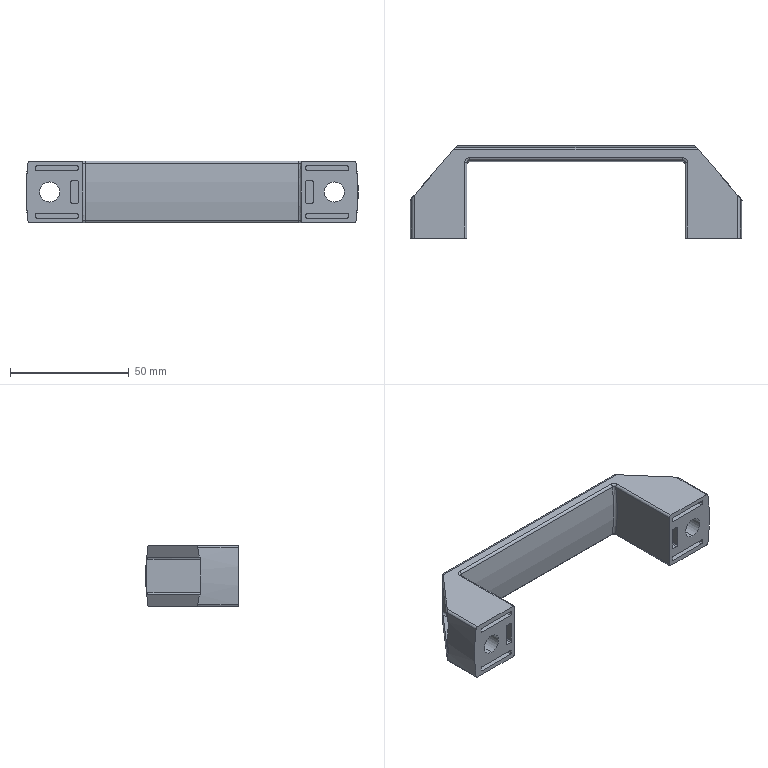Part | STEP file | XAP80-L120 | 1 solid | 106 faces | box 140 x 39 x 26 mm | volume 38026 mm3 | cylinder 52 | plane 48 | spline 6 | commonest cylinder face diameters 1 x24 2 x16 8.5 x4 14 x4 170 x4